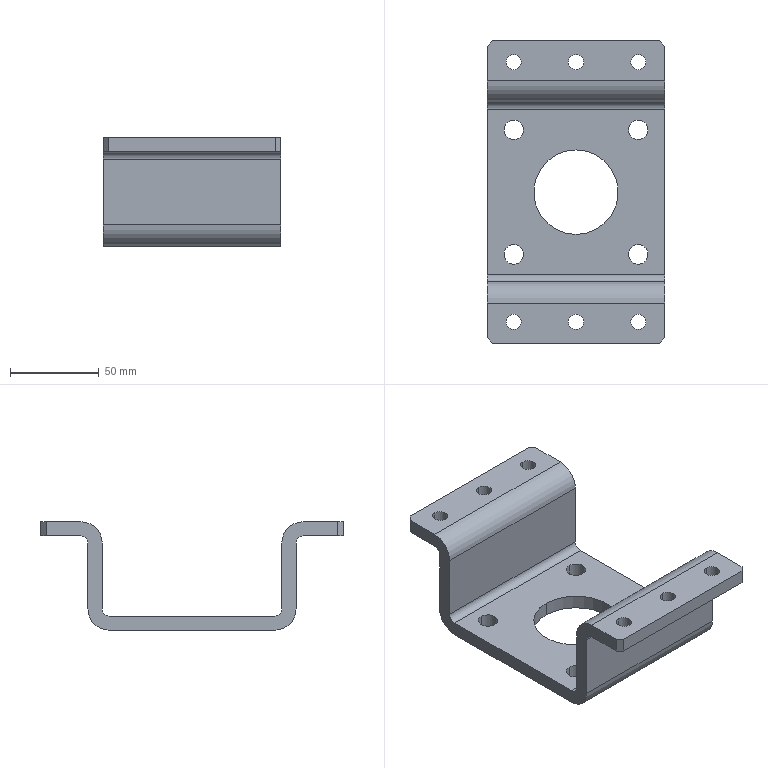Part | SolidWorks | features Fillet 2, HoleWzd 2, Chamfer 1, Extrusion 1, ICE 1 | 1 solid | 48 faces | box 100 x 170 x 61 mm | volume 189727 mm3 | cylinder 30 | plane 18 | commonest cylinder face diameters 8.5 x12 11 x8 8 x4 24 x4 47.5 x2